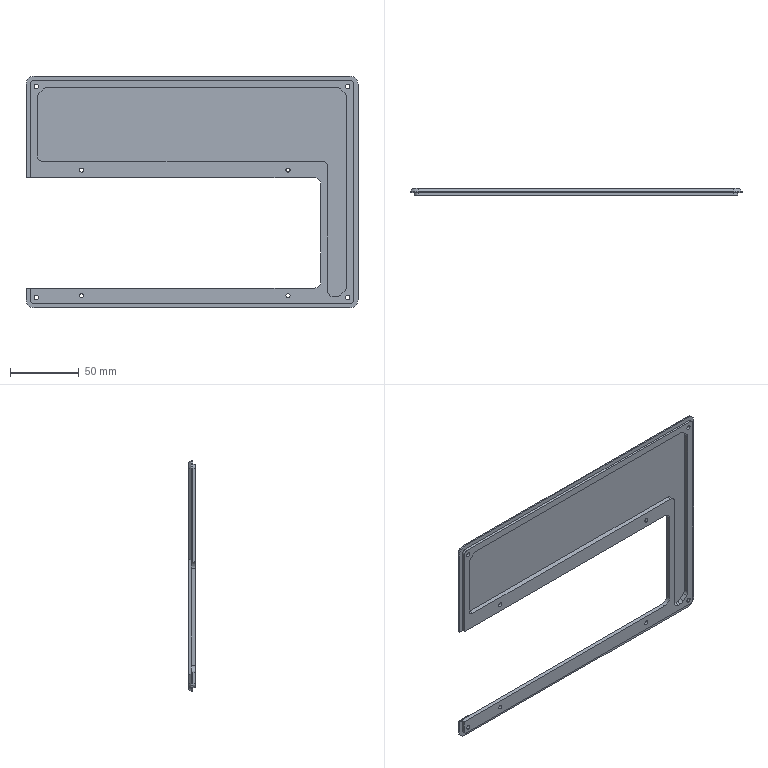NC program | NX | posted by the shop | part box 242 x 5 x 169 mm
Whole program:
%
(CUTTING TIME: 6.01)
(NAME: 2)
G17 G40 G49 G80 G90
G91 G28 Z0.
(TOOL_NAME :T3-D10-CX )
T03 M06
G00 G90 G54 X-127. Y-2.591 S6500 M03
G43 Z100. H03 M08 T06
G01 X-127. Y-2.591 Z-1.7 F5000.
G41 X-126.5 Y-2.6 F1500. D03
X-121. Y-2.6
X-110. Y-2.6
G02 X-97.577 Y-11.15 I0.0 J-13.3
G01 X86.2 Y-11.15
X86.2 Y70.75
X-97.577 Y70.75
G02 X-110. Y62.2 I-12.423 J4.75
G01 X-121. Y62.2
X-126.5 Y62.2
G40 X-127. Y62.191
X-127. Y-6.591
G41 X-126.5 Y-6.6
X-121. Y-6.6
X-110. Y-6.6
G02 X-100.73 Y-15.15 I0.0 J-9.3
G01 X90.2 Y-15.15
X90.2 Y74.75
X-100.73 Y74.75
G02 X-110. Y66.2 I-9.27 J.75
G01 X-121. Y66.2
X-126.5 Y66.2
G40 X-127. Y66.191
G00 Z100.
M05
M09
G91 G28 Z0.
M01
(TOOL_NAME :T6-D8-JX )
T06 M06
G00 G90 G54 X-125.9 Y-3.891 S6500 M03
G43 Z100. H06 M08 T03
G01 X-125.9 Y-3.891 Z-2. F5000.
G41 X-125.4 Y-3.9 F1500. D06
X-121. Y-3.9
X-110. Y-3.9
G02 X-98.507 Y-12.45 I0.0 J-12.
G01 X87.5 Y-12.45
X87.5 Y72.05
X-98.507 Y72.05
G02 X-110. Y63.5 I-11.493 J3.45
G01 X-121. Y63.5
X-125.4 Y63.5
G40 X-125.9 Y63.491
X-125.9 Y-7.891
G41 X-125.4 Y-7.9
X-121. Y-7.9
X-110. Y-7.9
G02 X-102. Y-15.9 I0.0 J-8.
G01 X-102. Y-16.45
X91.5 Y-16.45
X91.5 Y76.05
X-102. Y76.05
X-102. Y75.5
G02 X-110. Y67.5 I-8. J0.0
G01 X-121. Y67.5
X-125.4 Y67.5
G40 X-125.9 Y67.491
G00 Z100.
M05
M09
G91 G28 Z0.
M01
(TOOL_NAME :T3-D10-CX )
T03 M06
G00 G90 G54 X-131.711 Y-4.891 S6500 M03
G43 Z100. H03 M08 T04
G01 X-131.711 Y-4.891 Z-4.7 F5000.
G41 X-131.211 Y-4.9 F1500. D03
X-125.711 Y-4.9
X88.5 Y-4.9
X88.5 Y64.5
X-125.711 Y64.5
X-131.211 Y64.5
G40 X-131.711 Y64.491
G00 Z100.
M05
M09
G91 G28 Z0.
M01
M00-(Remove residual stock)
(TOOL_NAME :T4-D10-JX )
T04 M06
G00 G90 G54 X-131.711 Y-5.391 S6500 M03
G43 Z100. H04 M08 T10
G01 X-131.711 Y-5.391 Z-5.5 F5000.
G41 X-131.211 Y-5.4 F1500. D04
X-125.711 Y-5.4
X89. Y-5.4
X89. Y65.
X-125.711 Y65.
X-131.211 Y65.
G40 X-131.711 Y64.991
G00 Z100.
M05
M09
G91 G28 Z0.
M01
(TOOL_NAME :T10-D4-90° )
T10 M06
G00 G90 G54 X-121.7 Y-10.891 S6500 M03
G43 Z100. H10 M08 T09
G01 X-121.7 Y-10.891 Z-1. F5000.
G41 X-121.2 Y-10.9 F500.
X-119. Y-10.9
X-110. Y-10.9
G02 X-105. Y-15.9 I0.0 J-5.
G01 X-105. Y-16.45
G03 X-102. Y-19.45 I3. J0.0
G01 X91.5 Y-19.45
G03 X94.5 Y-16.45 I0.0 J3.
G01 X94.5 Y76.05
G03 X91.5 Y79.05 I-3. J0.0
G01 X-102. Y79.05
G03 X-105. Y76.05 I0.0 J-3.
G01 X-105. Y75.5
G02 X-110. Y70.5 I-5. J0.0
G01 X-119. Y70.5
X-121.2 Y70.5
G40 X-121.7 Y70.491
G00 Z100.
G00 G90 G54 X-123.7 Y-9.391 S6500 M03
G01 X-123.7 Y-9.391 Z-3. F5000.
G41 X-123.2 Y-9.4 F500.
X-121. Y-9.4
X89. Y-9.4
G03 X93. Y-5.4 I0.0 J4.
G01 X93. Y65.
G03 X89. Y69. I-4. J0.0
G01 X-121. Y69.
X-123.2 Y69.
G40 X-123.7 Y68.991
G00 Z100.
M05
M09
G91 G28 Z0.
M01
M00(Change clamp)
(TOOL_NAME :T9-D8-90° )
T09 M06
G00 G90 G54 X-124.646 Y63.181 S6500 M03
G43 Z103.146 H09 M08 T03
G01 X-124.646 Y63.181 Z.32 F5000.
X-124.646 Y63.181 Z-2.68 F500.
G03 X-121.675 Y67.105 I-1.028 J3.866
G01 X-121.681 Y67.522
X-121.68 Y78.602
G02 X-121.626 Y79.348 I6.68 J-.102
G01 X-121.513 Y79.987
G02 X-121.325 Y80.649 I6.513 J-1.487
G01 X-121.2 Y80.988
G02 X-121.111 Y81.199 I6.2 J-2.488
G01 X-121.082 Y81.263
X-121.056 Y81.321
X-120.997 Y81.443
G02 X-120.779 Y81.85 I5.997 J-2.943
G01 X-120.537 Y82.238
G02 X-120.392 Y82.444 I5.537 J-3.738
G01 X-120.315 Y82.547
G02 X-119.834 Y83.11 I5.315 J-4.047
G01 X-119.696 Y83.251
G02 X-119.502 Y83.435 I4.696 J-4.751
G01 X-119.424 Y83.505
G02 X-119.077 Y83.792 I4.424 J-5.005
G01 X-118.364 Y84.271
G02 X-117.97 Y84.484 I3.364 J-5.771
G01 X-117.72 Y84.602
X-117.553 Y84.674
X-117.191 Y84.811
G02 X-116.742 Y84.949 I2.191 J-6.311
G01 X-116.415 Y85.029
X-116.22 Y85.068
X-115.893 Y85.12
G02 X-115.445 Y85.166 I.893 J-6.62
G01 X115.414 Y85.168
G02 X115.861 Y85.125 I-.414 J-6.668
G01 X116.221 Y85.068
X116.416 Y85.029
X116.693 Y84.962
G02 X117.164 Y84.82 I-1.693 J-6.462
G01 X117.226 Y84.799
X117.345 Y84.755
X117.906 Y84.515
G02 X118.318 Y84.298 I-2.906 J-6.015
G01 X118.592 Y84.133
G02 X118.763 Y84.02 I-3.592 J-5.633
G01 X119.047 Y83.815
G02 X119.389 Y83.537 I-4.047 J-5.315
G01 X119.576 Y83.367
G02 X119.834 Y83.11 I-4.576 J-4.867
G01 X119.973 Y82.961
G02 X120.297 Y82.57 I-4.973 J-4.461
G01 X120.37 Y82.473
X120.429 Y82.393
X120.771 Y81.865
G02 X120.99 Y81.458 I-5.771 J-3.365
G01 X121.037 Y81.36
X121.082 Y81.263
X121.111 Y81.199
X121.184 Y81.026
X121.321 Y80.66
G02 X121.558 Y79.771 I-6.321 J-2.16
G01 X121.586 Y79.618
G02 X121.665 Y78.959 I-6.586 J-1.118
G01 X121.68 Y-78.602
G02 X121.627 Y-79.346 I-6.68 J.102
G01 X121.582 Y-79.642
G02 X121.184 Y-81.026 I-6.582 J1.142
G01 X121.025 Y-81.385
G02 X120.669 Y-82.035 I-6.025 J2.885
G01 X120.636 Y-82.086
X120.537 Y-82.238
X120.429 Y-82.393
X120.391 Y-82.445
X120.314 Y-82.548
G02 X119.973 Y-82.961 I-5.314 J4.048
G01 X119.834 Y-83.11
G02 X119.576 Y-83.367 I-4.834 J4.61
G01 X119.422 Y-83.507
G02 X119.077 Y-83.792 I-4.422 J5.007
G01 X118.875 Y-83.942
G02 X118.592 Y-84.133 I-3.875 J5.442
G01 X118.36 Y-84.274
G02 X117.97 Y-84.484 I-3.36 J5.774
G01 X117.898 Y-84.519
X117.345 Y-84.755
X117.276 Y-84.781
X117.191 Y-84.811
G02 X116.715 Y-84.956 I-2.191 J6.311
G01 X116.318 Y-85.049
X116.22 Y-85.068
X115.893 Y-85.12
G02 X115.447 Y-85.165 I-.893 J6.62
G01 X-115.413 Y-85.168
G02 X-115.859 Y-85.125 I.413 J6.668
G01 X-116.22 Y-85.068
X-116.415 Y-85.029
X-116.691 Y-84.963
G02 X-117.164 Y-84.82 I1.691 J6.463
G01 X-117.553 Y-84.674
X-117.72 Y-84.602
X-117.919 Y-84.509
G02 X-118.321 Y-84.296 I2.919 J6.009
G01 X-119.048 Y-83.814
G02 X-119.39 Y-83.535 I4.048 J5.314
G01 X-119.502 Y-83.435
G02 X-119.696 Y-83.251 I4.502 J4.935
G01 X-119.834 Y-83.11
G02 X-120.299 Y-82.568 I4.834 J4.61
G01 X-120.372 Y-82.472
X-120.433 Y-82.387
X-120.537 Y-82.238
X-120.64 Y-82.08
X-120.773 Y-81.861
G02 X-120.989 Y-81.459 I5.773 J3.361
G01 X-121.147 Y-81.116
X-121.184 Y-81.026
X-121.321 Y-80.663
G02 X-121.513 Y-79.988 I6.321 J2.163
G01 X-121.62 Y-79.395
G02 X-121.665 Y-78.955 I6.62 J.895
G01 X-121.68 Y-78.602
X-121.681 Y-7.964
X-121.676 Y-7.504
G03 X-124.654 Y-3.592 I-4. J.044
G01 X-124.654 Y-3.592 Z.32
G00 Z103.146
M05
M09
G91 G28 Z0.
G91 G28 Y0.
M30
%